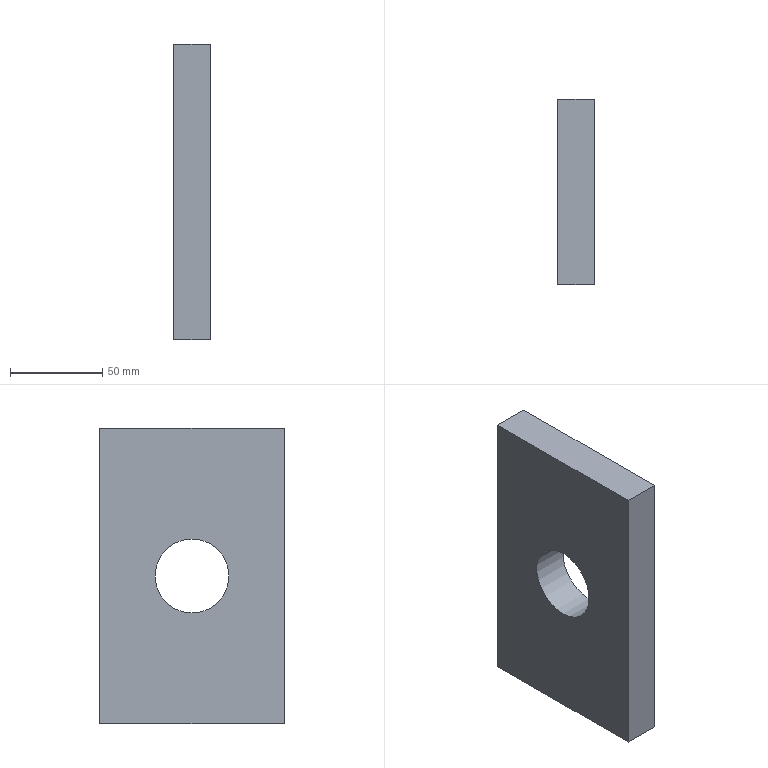Part | STEP file | Tube feed_id742_x_t | 1 solid | 7 faces | box 20 x 100 x 160 mm | volume 294867 mm3 | plane 6 | cylinder 1 | commonest cylinder face diameters 40 x1
STEP:
#1=CARTESIAN_POINT('',(0.,0.,0.));
#2=DIRECTION('',(0.,0.,1.));
#3=DIRECTION('',(1.,0.,0.));
#4=AXIS2_PLACEMENT_3D('',#1,#2,#3);
#5=CARTESIAN_POINT('',(326.,160.936,76.));
#6=VERTEX_POINT('',#5);
#7=CARTESIAN_POINT('',(326.,160.936,-84.));
#8=VERTEX_POINT('',#7);
#9=CARTESIAN_POINT('',(326.,160.936,76.));
#10=DIRECTION('',(0.,0.,-1.));
#11=VECTOR('',#10,1.);
#12=LINE('',#9,#11);
#13=CARTESIAN_POINT('',(346.,160.936,76.));
#14=DIRECTION('',(0.,1.,0.));
#15=DIRECTION('',(0.,0.,1.));
#16=AXIS2_PLACEMENT_3D('',#13,#14,#15);
#17=PLANE('',#16);
#18=CARTESIAN_POINT('',(0.,-20.));
#19=DIRECTION('',(-1.,0.));
#20=VECTOR('',#19,1.);
#21=LINE('',#18,#20);
#22=(GEOMETRIC_REPRESENTATION_CONTEXT(2)PARAMETRIC_REPRESENTATION_CONTEXT()REPRESENTATION_CONTEXT('',''));
#23=DEFINITIONAL_REPRESENTATION('',(#21),#22);
#24=PCURVE('',#17,#23);
#25=CARTESIAN_POINT('',(326.,0.,0.));
#26=DIRECTION('',(1.,0.,0.));
#27=DIRECTION('',(0.,0.,-1.));
#28=AXIS2_PLACEMENT_3D('',#25,#26,#27);
#29=PLANE('',#28);
#30=CARTESIAN_POINT('',(-76.,160.936));
#31=DIRECTION('',(1.,0.));
#32=VECTOR('',#31,1.);
#33=LINE('',#30,#32);
#34=(GEOMETRIC_REPRESENTATION_CONTEXT(2)PARAMETRIC_REPRESENTATION_CONTEXT()REPRESENTATION_CONTEXT('',''));
#35=DEFINITIONAL_REPRESENTATION('',(#33),#34);
#36=PCURVE('',#29,#35);
#37=SURFACE_CURVE('',#12,(#24,#36),.PCURVE_S1.);
#38=EDGE_CURVE('',#6,#8,#37,.T.);
#39=ORIENTED_EDGE('',*,*,#38,.T.);
#40=CARTESIAN_POINT('',(346.,160.936,-84.));
#41=VERTEX_POINT('',#40);
#42=CARTESIAN_POINT('',(346.,160.936,-84.));
#43=DIRECTION('',(-1.,0.,0.));
#44=VECTOR('',#43,1.);
#45=LINE('',#42,#44);
#46=CARTESIAN_POINT('',(-160.,0.));
#47=DIRECTION('',(0.,-1.));
#48=VECTOR('',#47,1.);
#49=LINE('',#46,#48);
#50=(GEOMETRIC_REPRESENTATION_CONTEXT(2)PARAMETRIC_REPRESENTATION_CONTEXT()REPRESENTATION_CONTEXT('',''));
#51=DEFINITIONAL_REPRESENTATION('',(#49),#50);
#52=PCURVE('',#17,#51);
#53=CARTESIAN_POINT('',(346.,160.936,-84.));
#54=DIRECTION('',(0.,0.,1.));
#55=DIRECTION('',(0.,-1.,0.));
#56=AXIS2_PLACEMENT_3D('',#53,#54,#55);
#57=PLANE('',#56);
#58=CARTESIAN_POINT('',(0.,0.));
#59=DIRECTION('',(0.,-1.));
#60=VECTOR('',#59,1.);
#61=LINE('',#58,#60);
#62=(GEOMETRIC_REPRESENTATION_CONTEXT(2)PARAMETRIC_REPRESENTATION_CONTEXT()REPRESENTATION_CONTEXT('',''));
#63=DEFINITIONAL_REPRESENTATION('',(#61),#62);
#64=PCURVE('',#57,#63);
#65=SURFACE_CURVE('',#45,(#52,#64),.PCURVE_S1.);
#66=EDGE_CURVE('',#41,#8,#65,.T.);
#67=ORIENTED_EDGE('',*,*,#66,.F.);
#68=CARTESIAN_POINT('',(346.,160.936,76.));
#69=VERTEX_POINT('',#68);
#70=CARTESIAN_POINT('',(346.,160.936,76.));
#71=DIRECTION('',(0.,0.,-1.));
#72=VECTOR('',#71,1.);
#73=LINE('',#70,#72);
#74=CARTESIAN_POINT('',(0.,0.));
#75=DIRECTION('',(-1.,0.));
#76=VECTOR('',#75,1.);
#77=LINE('',#74,#76);
#78=(GEOMETRIC_REPRESENTATION_CONTEXT(2)PARAMETRIC_REPRESENTATION_CONTEXT()REPRESENTATION_CONTEXT('',''));
#79=DEFINITIONAL_REPRESENTATION('',(#77),#78);
#80=PCURVE('',#17,#79);
#81=CARTESIAN_POINT('',(346.,0.,0.));
#82=DIRECTION('',(1.,0.,0.));
#83=DIRECTION('',(0.,0.,-1.));
#84=AXIS2_PLACEMENT_3D('',#81,#82,#83);
#85=PLANE('',#84);
#86=CARTESIAN_POINT('',(-76.,160.936));
#87=DIRECTION('',(1.,0.));
#88=VECTOR('',#87,1.);
#89=LINE('',#86,#88);
#90=(GEOMETRIC_REPRESENTATION_CONTEXT(2)PARAMETRIC_REPRESENTATION_CONTEXT()REPRESENTATION_CONTEXT('',''));
#91=DEFINITIONAL_REPRESENTATION('',(#89),#90);
#92=PCURVE('',#85,#91);
#93=SURFACE_CURVE('',#73,(#80,#92),.PCURVE_S1.);
#94=EDGE_CURVE('',#69,#41,#93,.T.);
#95=ORIENTED_EDGE('',*,*,#94,.F.);
#96=CARTESIAN_POINT('',(346.,160.936,76.));
#97=DIRECTION('',(-1.,0.,0.));
#98=VECTOR('',#97,1.);
#99=LINE('',#96,#98);
#100=CARTESIAN_POINT('',(0.,0.));
#101=DIRECTION('',(0.,-1.));
#102=VECTOR('',#101,1.);
#103=LINE('',#100,#102);
#104=(GEOMETRIC_REPRESENTATION_CONTEXT(2)PARAMETRIC_REPRESENTATION_CONTEXT()REPRESENTATION_CONTEXT('',''));
#105=DEFINITIONAL_REPRESENTATION('',(#103),#104);
#106=PCURVE('',#17,#105);
#107=CARTESIAN_POINT('',(346.,260.936,76.));
#108=DIRECTION('',(0.,0.,-1.));
#109=DIRECTION('',(0.,1.,0.));
#110=AXIS2_PLACEMENT_3D('',#107,#108,#109);
#111=PLANE('',#110);
#112=CARTESIAN_POINT('',(-100.,0.));
#113=DIRECTION('',(0.,-1.));
#114=VECTOR('',#113,1.);
#115=LINE('',#112,#114);
#116=(GEOMETRIC_REPRESENTATION_CONTEXT(2)PARAMETRIC_REPRESENTATION_CONTEXT()REPRESENTATION_CONTEXT('',''));
#117=DEFINITIONAL_REPRESENTATION('',(#115),#116);
#118=PCURVE('',#111,#117);
#119=SURFACE_CURVE('',#99,(#106,#118),.PCURVE_S1.);
#120=EDGE_CURVE('',#69,#6,#119,.T.);
#121=ORIENTED_EDGE('',*,*,#120,.T.);
#122=EDGE_LOOP('',(#39,#67,#95,#121));
#123=FACE_BOUND('',#122,.T.);
#124=ADVANCED_FACE('',(#123),#17,.F.);
#125=CARTESIAN_POINT('',(326.,260.936,-84.));
#126=VERTEX_POINT('',#125);
#127=CARTESIAN_POINT('',(326.,160.936,-84.));
#128=DIRECTION('',(0.,1.,0.));
#129=VECTOR('',#128,1.);
#130=LINE('',#127,#129);
#131=CARTESIAN_POINT('',(0.,-20.));
#132=DIRECTION('',(-1.,0.));
#133=VECTOR('',#132,1.);
#134=LINE('',#131,#133);
#135=(GEOMETRIC_REPRESENTATION_CONTEXT(2)PARAMETRIC_REPRESENTATION_CONTEXT()REPRESENTATION_CONTEXT('',''));
#136=DEFINITIONAL_REPRESENTATION('',(#134),#135);
#137=PCURVE('',#57,#136);
#138=CARTESIAN_POINT('',(84.,160.936));
#139=DIRECTION('',(0.,1.));
#140=VECTOR('',#139,1.);
#141=LINE('',#138,#140);
#142=(GEOMETRIC_REPRESENTATION_CONTEXT(2)PARAMETRIC_REPRESENTATION_CONTEXT()REPRESENTATION_CONTEXT('',''));
#143=DEFINITIONAL_REPRESENTATION('',(#141),#142);
#144=PCURVE('',#29,#143);
#145=SURFACE_CURVE('',#130,(#137,#144),.PCURVE_S1.);
#146=EDGE_CURVE('',#8,#126,#145,.T.);
#147=ORIENTED_EDGE('',*,*,#146,.T.);
#148=CARTESIAN_POINT('',(346.,260.936,-84.));
#149=VERTEX_POINT('',#148);
#150=CARTESIAN_POINT('',(346.,260.936,-84.));
#151=DIRECTION('',(-1.,0.,0.));
#152=VECTOR('',#151,1.);
#153=LINE('',#150,#152);
#154=CARTESIAN_POINT('',(-100.,0.));
#155=DIRECTION('',(0.,-1.));
#156=VECTOR('',#155,1.);
#157=LINE('',#154,#156);
#158=(GEOMETRIC_REPRESENTATION_CONTEXT(2)PARAMETRIC_REPRESENTATION_CONTEXT()REPRESENTATION_CONTEXT('',''));
#159=DEFINITIONAL_REPRESENTATION('',(#157),#158);
#160=PCURVE('',#57,#159);
#161=CARTESIAN_POINT('',(346.,260.936,-84.));
#162=DIRECTION('',(0.,-1.,0.));
#163=DIRECTION('',(0.,0.,-1.));
#164=AXIS2_PLACEMENT_3D('',#161,#162,#163);
#165=PLANE('',#164);
#166=CARTESIAN_POINT('',(0.,0.));
#167=DIRECTION('',(0.,-1.));
#168=VECTOR('',#167,1.);
#169=LINE('',#166,#168);
#170=(GEOMETRIC_REPRESENTATION_CONTEXT(2)PARAMETRIC_REPRESENTATION_CONTEXT()REPRESENTATION_CONTEXT('',''));
#171=DEFINITIONAL_REPRESENTATION('',(#169),#170);
#172=PCURVE('',#165,#171);
#173=SURFACE_CURVE('',#153,(#160,#172),.PCURVE_S1.);
#174=EDGE_CURVE('',#149,#126,#173,.T.);
#175=ORIENTED_EDGE('',*,*,#174,.F.);
#176=CARTESIAN_POINT('',(346.,160.936,-84.));
#177=DIRECTION('',(0.,1.,0.));
#178=VECTOR('',#177,1.);
#179=LINE('',#176,#178);
#180=CARTESIAN_POINT('',(0.,0.));
#181=DIRECTION('',(-1.,0.));
#182=VECTOR('',#181,1.);
#183=LINE('',#180,#182);
#184=(GEOMETRIC_REPRESENTATION_CONTEXT(2)PARAMETRIC_REPRESENTATION_CONTEXT()REPRESENTATION_CONTEXT('',''));
#185=DEFINITIONAL_REPRESENTATION('',(#183),#184);
#186=PCURVE('',#57,#185);
#187=CARTESIAN_POINT('',(84.,160.936));
#188=DIRECTION('',(0.,1.));
#189=VECTOR('',#188,1.);
#190=LINE('',#187,#189);
#191=(GEOMETRIC_REPRESENTATION_CONTEXT(2)PARAMETRIC_REPRESENTATION_CONTEXT()REPRESENTATION_CONTEXT('',''));
#192=DEFINITIONAL_REPRESENTATION('',(#190),#191);
#193=PCURVE('',#85,#192);
#194=SURFACE_CURVE('',#179,(#186,#193),.PCURVE_S1.);
#195=EDGE_CURVE('',#41,#149,#194,.T.);
#196=ORIENTED_EDGE('',*,*,#195,.F.);
#197=ORIENTED_EDGE('',*,*,#66,.T.);
#198=EDGE_LOOP('',(#147,#175,#196,#197));
#199=FACE_BOUND('',#198,.T.);
#200=ADVANCED_FACE('',(#199),#57,.F.);
#201=CARTESIAN_POINT('',(326.,260.936,76.));
#202=VERTEX_POINT('',#201);
#203=CARTESIAN_POINT('',(326.,260.936,-84.));
#204=DIRECTION('',(0.,0.,1.));
#205=VECTOR('',#204,1.);
#206=LINE('',#203,#205);
#207=CARTESIAN_POINT('',(0.,-20.));
#208=DIRECTION('',(-1.,0.));
#209=VECTOR('',#208,1.);
#210=LINE('',#207,#209);
#211=(GEOMETRIC_REPRESENTATION_CONTEXT(2)PARAMETRIC_REPRESENTATION_CONTEXT()REPRESENTATION_CONTEXT('',''));
#212=DEFINITIONAL_REPRESENTATION('',(#210),#211);
#213=PCURVE('',#165,#212);
#214=CARTESIAN_POINT('',(84.,260.936));
#215=DIRECTION('',(-1.,0.));
#216=VECTOR('',#215,1.);
#217=LINE('',#214,#216);
#218=(GEOMETRIC_REPRESENTATION_CONTEXT(2)PARAMETRIC_REPRESENTATION_CONTEXT()REPRESENTATION_CONTEXT('',''));
#219=DEFINITIONAL_REPRESENTATION('',(#217),#218);
#220=PCURVE('',#29,#219);
#221=SURFACE_CURVE('',#206,(#213,#220),.PCURVE_S1.);
#222=EDGE_CURVE('',#126,#202,#221,.T.);
#223=ORIENTED_EDGE('',*,*,#222,.T.);
#224=CARTESIAN_POINT('',(346.,260.936,76.));
#225=VERTEX_POINT('',#224);
#226=CARTESIAN_POINT('',(346.,260.936,76.));
#227=DIRECTION('',(-1.,0.,0.));
#228=VECTOR('',#227,1.);
#229=LINE('',#226,#228);
#230=CARTESIAN_POINT('',(-160.,0.));
#231=DIRECTION('',(0.,-1.));
#232=VECTOR('',#231,1.);
#233=LINE('',#230,#232);
#234=(GEOMETRIC_REPRESENTATION_CONTEXT(2)PARAMETRIC_REPRESENTATION_CONTEXT()REPRESENTATION_CONTEXT('',''));
#235=DEFINITIONAL_REPRESENTATION('',(#233),#234);
#236=PCURVE('',#165,#235);
#237=CARTESIAN_POINT('',(0.,0.));
#238=DIRECTION('',(0.,-1.));
#239=VECTOR('',#238,1.);
#240=LINE('',#237,#239);
#241=(GEOMETRIC_REPRESENTATION_CONTEXT(2)PARAMETRIC_REPRESENTATION_CONTEXT()REPRESENTATION_CONTEXT('',''));
#242=DEFINITIONAL_REPRESENTATION('',(#240),#241);
#243=PCURVE('',#111,#242);
#244=SURFACE_CURVE('',#229,(#236,#243),.PCURVE_S1.);
#245=EDGE_CURVE('',#225,#202,#244,.T.);
#246=ORIENTED_EDGE('',*,*,#245,.F.);
#247=CARTESIAN_POINT('',(346.,260.936,-84.));
#248=DIRECTION('',(0.,0.,1.));
#249=VECTOR('',#248,1.);
#250=LINE('',#247,#249);
#251=CARTESIAN_POINT('',(0.,0.));
#252=DIRECTION('',(-1.,0.));
#253=VECTOR('',#252,1.);
#254=LINE('',#251,#253);
#255=(GEOMETRIC_REPRESENTATION_CONTEXT(2)PARAMETRIC_REPRESENTATION_CONTEXT()REPRESENTATION_CONTEXT('',''));
#256=DEFINITIONAL_REPRESENTATION('',(#254),#255);
#257=PCURVE('',#165,#256);
#258=CARTESIAN_POINT('',(84.,260.936));
#259=DIRECTION('',(-1.,0.));
#260=VECTOR('',#259,1.);
#261=LINE('',#258,#260);
#262=(GEOMETRIC_REPRESENTATION_CONTEXT(2)PARAMETRIC_REPRESENTATION_CONTEXT()REPRESENTATION_CONTEXT('',''));
#263=DEFINITIONAL_REPRESENTATION('',(#261),#262);
#264=PCURVE('',#85,#263);
#265=SURFACE_CURVE('',#250,(#257,#264),.PCURVE_S1.);
#266=EDGE_CURVE('',#149,#225,#265,.T.);
#267=ORIENTED_EDGE('',*,*,#266,.F.);
#268=ORIENTED_EDGE('',*,*,#174,.T.);
#269=EDGE_LOOP('',(#223,#246,#267,#268));
#270=FACE_BOUND('',#269,.T.);
#271=ADVANCED_FACE('',(#270),#165,.F.);
#272=CARTESIAN_POINT('',(326.,260.936,76.));
#273=DIRECTION('',(0.,-1.,0.));
#274=VECTOR('',#273,1.);
#275=LINE('',#272,#274);
#276=CARTESIAN_POINT('',(0.,-20.));
#277=DIRECTION('',(-1.,0.));
#278=VECTOR('',#277,1.);
#279=LINE('',#276,#278);
#280=(GEOMETRIC_REPRESENTATION_CONTEXT(2)PARAMETRIC_REPRESENTATION_CONTEXT()REPRESENTATION_CONTEXT('',''));
#281=DEFINITIONAL_REPRESENTATION('',(#279),#280);
#282=PCURVE('',#111,#281);
#283=CARTESIAN_POINT('',(-76.,260.936));
#284=DIRECTION('',(0.,-1.));
#285=VECTOR('',#284,1.);
#286=LINE('',#283,#285);
#287=(GEOMETRIC_REPRESENTATION_CONTEXT(2)PARAMETRIC_REPRESENTATION_CONTEXT()REPRESENTATION_CONTEXT('',''));
#288=DEFINITIONAL_REPRESENTATION('',(#286),#287);
#289=PCURVE('',#29,#288);
#290=SURFACE_CURVE('',#275,(#282,#289),.PCURVE_S1.);
#291=EDGE_CURVE('',#202,#6,#290,.T.);
#292=ORIENTED_EDGE('',*,*,#291,.T.);
#293=ORIENTED_EDGE('',*,*,#120,.F.);
#294=CARTESIAN_POINT('',(346.,260.936,76.));
#295=DIRECTION('',(0.,-1.,0.));
#296=VECTOR('',#295,1.);
#297=LINE('',#294,#296);
#298=CARTESIAN_POINT('',(0.,0.));
#299=DIRECTION('',(-1.,0.));
#300=VECTOR('',#299,1.);
#301=LINE('',#298,#300);
#302=(GEOMETRIC_REPRESENTATION_CONTEXT(2)PARAMETRIC_REPRESENTATION_CONTEXT()REPRESENTATION_CONTEXT('',''));
#303=DEFINITIONAL_REPRESENTATION('',(#301),#302);
#304=PCURVE('',#111,#303);
#305=CARTESIAN_POINT('',(-76.,260.936));
#306=DIRECTION('',(0.,-1.));
#307=VECTOR('',#306,1.);
#308=LINE('',#305,#307);
#309=(GEOMETRIC_REPRESENTATION_CONTEXT(2)PARAMETRIC_REPRESENTATION_CONTEXT()REPRESENTATION_CONTEXT('',''));
#310=DEFINITIONAL_REPRESENTATION('',(#308),#309);
#311=PCURVE('',#85,#310);
#312=SURFACE_CURVE('',#297,(#304,#311),.PCURVE_S1.);
#313=EDGE_CURVE('',#225,#69,#312,.T.);
#314=ORIENTED_EDGE('',*,*,#313,.F.);
#315=ORIENTED_EDGE('',*,*,#245,.T.);
#316=EDGE_LOOP('',(#292,#293,#314,#315));
#317=FACE_BOUND('',#316,.T.);
#318=ADVANCED_FACE('',(#317),#111,.F.);
#319=CARTESIAN_POINT('',(346.,210.936,-24.));
#320=VERTEX_POINT('',#319);
#321=CARTESIAN_POINT('',(346.,210.936,-4.));
#322=DIRECTION('',(-1.,0.,0.));
#323=DIRECTION('',(0.,0.,-1.));
#324=AXIS2_PLACEMENT_3D('',#321,#322,#323);
#325=CIRCLE('',#324,20.);
#326=CARTESIAN_POINT('',(24.,210.936));
#327=CARTESIAN_POINT('',(24.,176.295));
#328=CARTESIAN_POINT('',(-6.,193.615));
#329=CARTESIAN_POINT('',(-36.,210.936));
#330=CARTESIAN_POINT('',(-6.,228.256));
#331=CARTESIAN_POINT('',(24.,245.577));
#332=CARTESIAN_POINT('',(24.,210.936));
#333=(BOUNDED_CURVE()B_SPLINE_CURVE(2,(#326,#327,#328,#329,#330,#331,#332),.UNSPECIFIED.,.T.,.F.)B_SPLINE_CURVE_WITH_KNOTS((1,2,2,2,2,1),(-2.094,0.,2.094,4.189,6.283,8.378),.UNSPECIFIED.)CURVE()GEOMETRIC_REPRESENTATION_ITEM()RATIONAL_B_SPLINE_CURVE((1.,0.5,1.,0.5,1.,0.5,1.))REPRESENTATION_ITEM(''));
#334=(GEOMETRIC_REPRESENTATION_CONTEXT(2)PARAMETRIC_REPRESENTATION_CONTEXT()REPRESENTATION_CONTEXT('',''));
#335=DEFINITIONAL_REPRESENTATION('',(#333),#334);
#336=PCURVE('',#85,#335);
#337=CARTESIAN_POINT('',(375.,210.936,-4.));
#338=DIRECTION('',(-1.,0.,0.));
#339=DIRECTION('',(0.,0.,1.));
#340=AXIS2_PLACEMENT_3D('',#337,#338,#339);
#341=CYLINDRICAL_SURFACE('',#340,20.);
#342=CARTESIAN_POINT('',(3.142,29.));
#343=DIRECTION('',(1.,0.));
#344=VECTOR('',#343,1.);
#345=LINE('',#342,#344);
#346=(GEOMETRIC_REPRESENTATION_CONTEXT(2)PARAMETRIC_REPRESENTATION_CONTEXT()REPRESENTATION_CONTEXT('',''));
#347=DEFINITIONAL_REPRESENTATION('',(#345),#346);
#348=PCURVE('',#341,#347);
#349=SURFACE_CURVE('',#325,(#336,#348),.PCURVE_S1.);
#350=EDGE_CURVE('',#320,#320,#349,.T.);
#351=ORIENTED_EDGE('',*,*,#350,.T.);
#352=EDGE_LOOP('',(#351));
#353=FACE_BOUND('',#352,.T.);
#354=ORIENTED_EDGE('',*,*,#94,.T.);
#355=ORIENTED_EDGE('',*,*,#195,.T.);
#356=ORIENTED_EDGE('',*,*,#266,.T.);
#357=ORIENTED_EDGE('',*,*,#313,.T.);
#358=EDGE_LOOP('',(#354,#355,#356,#357));
#359=FACE_BOUND('',#358,.T.);
#360=ADVANCED_FACE('',(#353,#359),#85,.T.);
#361=CARTESIAN_POINT('',(326.,210.936,-24.));
#362=VERTEX_POINT('',#361);
#363=CARTESIAN_POINT('',(326.,210.936,-4.));
#364=DIRECTION('',(-1.,0.,0.));
#365=DIRECTION('',(0.,0.,-1.));
#366=AXIS2_PLACEMENT_3D('',#363,#364,#365);
#367=CIRCLE('',#366,20.);
#368=CARTESIAN_POINT('',(24.,210.936));
#369=CARTESIAN_POINT('',(24.,176.295));
#370=CARTESIAN_POINT('',(-6.,193.615));
#371=CARTESIAN_POINT('',(-36.,210.936));
#372=CARTESIAN_POINT('',(-6.,228.256));
#373=CARTESIAN_POINT('',(24.,245.577));
#374=CARTESIAN_POINT('',(24.,210.936));
#375=(BOUNDED_CURVE()B_SPLINE_CURVE(2,(#368,#369,#370,#371,#372,#373,#374),.UNSPECIFIED.,.T.,.F.)B_SPLINE_CURVE_WITH_KNOTS((1,2,2,2,2,1),(-2.094,0.,2.094,4.189,6.283,8.378),.UNSPECIFIED.)CURVE()GEOMETRIC_REPRESENTATION_ITEM()RATIONAL_B_SPLINE_CURVE((1.,0.5,1.,0.5,1.,0.5,1.))REPRESENTATION_ITEM(''));
#376=(GEOMETRIC_REPRESENTATION_CONTEXT(2)PARAMETRIC_REPRESENTATION_CONTEXT()REPRESENTATION_CONTEXT('',''));
#377=DEFINITIONAL_REPRESENTATION('',(#375),#376);
#378=PCURVE('',#29,#377);
#379=CARTESIAN_POINT('',(3.142,49.));
#380=DIRECTION('',(1.,0.));
#381=VECTOR('',#380,1.);
#382=LINE('',#379,#381);
#383=(GEOMETRIC_REPRESENTATION_CONTEXT(2)PARAMETRIC_REPRESENTATION_CONTEXT()REPRESENTATION_CONTEXT('',''));
#384=DEFINITIONAL_REPRESENTATION('',(#382),#383);
#385=PCURVE('',#341,#384);
#386=SURFACE_CURVE('',#367,(#378,#385),.PCURVE_S1.);
#387=EDGE_CURVE('',#362,#362,#386,.T.);
#388=ORIENTED_EDGE('',*,*,#387,.F.);
#389=EDGE_LOOP('',(#388));
#390=FACE_BOUND('',#389,.T.);
#391=ORIENTED_EDGE('',*,*,#38,.F.);
#392=ORIENTED_EDGE('',*,*,#291,.F.);
#393=ORIENTED_EDGE('',*,*,#222,.F.);
#394=ORIENTED_EDGE('',*,*,#146,.F.);
#395=EDGE_LOOP('',(#391,#392,#393,#394));
#396=FACE_BOUND('',#395,.T.);
#397=ADVANCED_FACE('',(#390,#396),#29,.F.);
#398=ORIENTED_EDGE('',*,*,#350,.T.);
#399=CARTESIAN_POINT('',(346.,210.936,-24.));
#400=CARTESIAN_POINT('',(326.,210.936,-24.));
#401=B_SPLINE_CURVE_WITH_KNOTS('',1,(#399,#400),.UNSPECIFIED.,.F.,.F.,(2,2),(29.,49.),.PIECEWISE_BEZIER_KNOTS.);
#402=CARTESIAN_POINT('',(9.425,0.));
#403=DIRECTION('',(0.,1.));
#404=VECTOR('',#403,1.);
#405=LINE('',#402,#404);
#406=(GEOMETRIC_REPRESENTATION_CONTEXT(2)PARAMETRIC_REPRESENTATION_CONTEXT()REPRESENTATION_CONTEXT('',''));
#407=DEFINITIONAL_REPRESENTATION('',(#405),#406);
#408=PCURVE('',#341,#407);
#409=CARTESIAN_POINT('',(3.142,0.));
#410=DIRECTION('',(0.,1.));
#411=VECTOR('',#410,1.);
#412=LINE('',#409,#411);
#413=(GEOMETRIC_REPRESENTATION_CONTEXT(2)PARAMETRIC_REPRESENTATION_CONTEXT()REPRESENTATION_CONTEXT('',''));
#414=DEFINITIONAL_REPRESENTATION('',(#412),#413);
#415=PCURVE('',#341,#414);
#416=SEAM_CURVE('',#401,(#408,#415),.PCURVE_S1.);
#417=EDGE_CURVE('',#320,#362,#416,.T.);
#418=ORIENTED_EDGE('',*,*,#417,.T.);
#419=ORIENTED_EDGE('',*,*,#387,.F.);
#420=ORIENTED_EDGE('',*,*,#417,.F.);
#421=EDGE_LOOP('',(#398,#418,#419,#420));
#422=FACE_BOUND('',#421,.F.);
#423=ADVANCED_FACE('',(#422),#341,.F.);
#424=CLOSED_SHELL('',(#124,#200,#271,#318,#360,#397,#423));
#425=MANIFOLD_SOLID_BREP('',#424);
#426=(LENGTH_UNIT()NAMED_UNIT(*)SI_UNIT(.MILLI.,.METRE.));
#427=UNCERTAINTY_MEASURE_WITH_UNIT(LENGTH_MEASURE(0.000002),#426,'','');
#428=(NAMED_UNIT(*)PLANE_ANGLE_UNIT()SI_UNIT($,.RADIAN.));
#429=(NAMED_UNIT(*)SI_UNIT($,.STERADIAN.)SOLID_ANGLE_UNIT());
#430=(GEOMETRIC_REPRESENTATION_CONTEXT(3)GLOBAL_UNCERTAINTY_ASSIGNED_CONTEXT((#427))GLOBAL_UNIT_ASSIGNED_CONTEXT((#426,#428,#429))REPRESENTATION_CONTEXT('',''));
#431=ADVANCED_BREP_SHAPE_REPRESENTATION('',(#4,#425),#430);